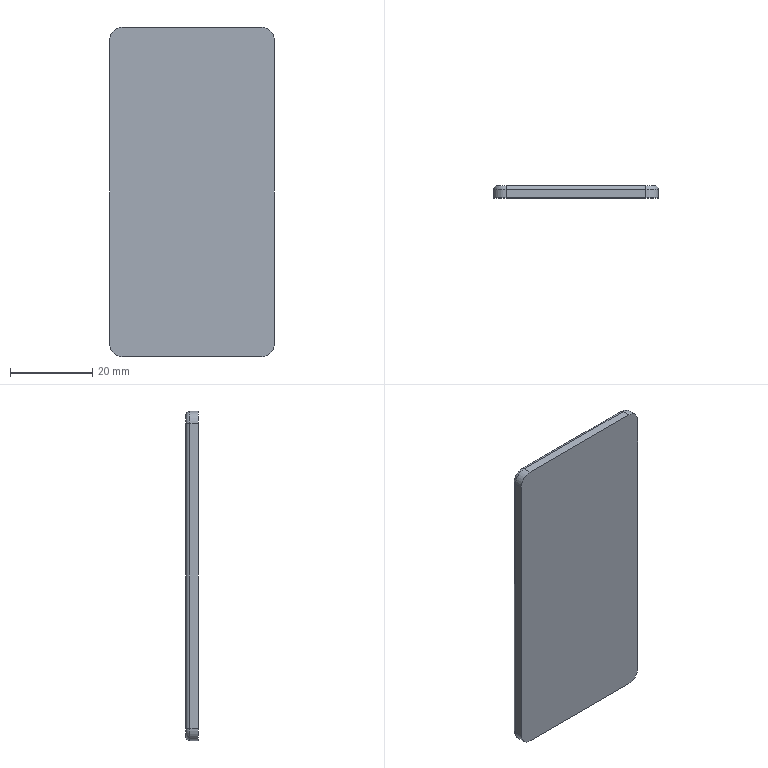Part | SolidWorks | features Fillet 2, Extrusion 1 | 1 solid | 18 faces | box 40 x 3 x 80 mm | volume 9527 mm3 | cylinder 8 | plane 6 | torus 4 | commonest cylinder face diameters 2 x4 6 x4
STEP:
#1=CARTESIAN_POINT('',(20.,0.,-37.));
#2=VERTEX_POINT('',#1);
#3=CARTESIAN_POINT('',(20.,2.,-37.));
#4=VERTEX_POINT('',#3);
#5=CARTESIAN_POINT('',(20.,3.,-37.));
#6=DIRECTION('',(0.,1.,0.));
#7=VECTOR('',#6,1000.);
#8=LINE('',#5,#7);
#9=EDGE_CURVE('',#2,#4,#8,.T.);
#10=ORIENTED_EDGE('',*,*,#9,.T.);
#11=CARTESIAN_POINT('',(20.,2.,37.));
#12=VERTEX_POINT('',#11);
#13=CARTESIAN_POINT('',(20.,2.,40.));
#14=DIRECTION('',(0.,0.,1.));
#15=VECTOR('',#14,1000.);
#16=LINE('',#13,#15);
#17=EDGE_CURVE('',#4,#12,#16,.T.);
#18=ORIENTED_EDGE('',*,*,#17,.T.);
#19=CARTESIAN_POINT('',(20.,0.,37.));
#20=VERTEX_POINT('',#19);
#21=CARTESIAN_POINT('',(20.,3.,37.));
#22=DIRECTION('',(0.,-1.,0.));
#23=VECTOR('',#22,1000.);
#24=LINE('',#21,#23);
#25=EDGE_CURVE('',#12,#20,#24,.T.);
#26=ORIENTED_EDGE('',*,*,#25,.T.);
#27=CARTESIAN_POINT('',(20.,0.,40.));
#28=DIRECTION('',(0.,0.,-1.));
#29=VECTOR('',#28,1000.);
#30=LINE('',#27,#29);
#31=EDGE_CURVE('',#20,#2,#30,.T.);
#32=ORIENTED_EDGE('',*,*,#31,.T.);
#33=EDGE_LOOP('',(#10,#18,#26,#32));
#34=FACE_OUTER_BOUND('',#33,.T.);
#35=CARTESIAN_POINT('',(20.,3.,40.));
#36=DIRECTION('',(-1.,0.,0.));
#37=DIRECTION('',(0.,0.,1.));
#38=AXIS2_PLACEMENT_3D('',#35,#36,#37);
#39=PLANE('',#38);
#40=ADVANCED_FACE('',(#34),#39,.F.);
#41=CARTESIAN_POINT('',(-17.,0.,-40.));
#42=VERTEX_POINT('',#41);
#43=CARTESIAN_POINT('',(-17.,2.,-40.));
#44=VERTEX_POINT('',#43);
#45=CARTESIAN_POINT('',(-17.,3.,-40.));
#46=DIRECTION('',(0.,1.,0.));
#47=VECTOR('',#46,1000.);
#48=LINE('',#45,#47);
#49=EDGE_CURVE('',#42,#44,#48,.T.);
#50=ORIENTED_EDGE('',*,*,#49,.T.);
#51=CARTESIAN_POINT('',(17.,2.,-40.));
#52=VERTEX_POINT('',#51);
#53=CARTESIAN_POINT('',(-20.,2.,-40.));
#54=DIRECTION('',(1.,0.,0.));
#55=VECTOR('',#54,1000.);
#56=LINE('',#53,#55);
#57=EDGE_CURVE('',#44,#52,#56,.T.);
#58=ORIENTED_EDGE('',*,*,#57,.T.);
#59=CARTESIAN_POINT('',(17.,0.,-40.));
#60=VERTEX_POINT('',#59);
#61=CARTESIAN_POINT('',(17.,3.,-40.));
#62=DIRECTION('',(0.,-1.,0.));
#63=VECTOR('',#62,1000.);
#64=LINE('',#61,#63);
#65=EDGE_CURVE('',#52,#60,#64,.T.);
#66=ORIENTED_EDGE('',*,*,#65,.T.);
#67=CARTESIAN_POINT('',(-20.,0.,-40.));
#68=DIRECTION('',(-1.,0.,0.));
#69=VECTOR('',#68,1000.);
#70=LINE('',#67,#69);
#71=EDGE_CURVE('',#60,#42,#70,.T.);
#72=ORIENTED_EDGE('',*,*,#71,.T.);
#73=EDGE_LOOP('',(#50,#58,#66,#72));
#74=FACE_OUTER_BOUND('',#73,.T.);
#75=CARTESIAN_POINT('',(-20.,3.,-40.));
#76=DIRECTION('',(0.,0.,1.));
#77=DIRECTION('',(1.,0.,0.));
#78=AXIS2_PLACEMENT_3D('',#75,#76,#77);
#79=PLANE('',#78);
#80=ADVANCED_FACE('',(#74),#79,.F.);
#81=CARTESIAN_POINT('',(-20.,0.,37.));
#82=VERTEX_POINT('',#81);
#83=CARTESIAN_POINT('',(-20.,2.,37.));
#84=VERTEX_POINT('',#83);
#85=CARTESIAN_POINT('',(-20.,3.,37.));
#86=DIRECTION('',(0.,1.,0.));
#87=VECTOR('',#86,1000.);
#88=LINE('',#85,#87);
#89=EDGE_CURVE('',#82,#84,#88,.T.);
#90=ORIENTED_EDGE('',*,*,#89,.T.);
#91=CARTESIAN_POINT('',(-20.,2.,-37.));
#92=VERTEX_POINT('',#91);
#93=CARTESIAN_POINT('',(-20.,2.,40.));
#94=DIRECTION('',(0.,0.,-1.));
#95=VECTOR('',#94,1000.);
#96=LINE('',#93,#95);
#97=EDGE_CURVE('',#84,#92,#96,.T.);
#98=ORIENTED_EDGE('',*,*,#97,.T.);
#99=CARTESIAN_POINT('',(-20.,0.,-37.));
#100=VERTEX_POINT('',#99);
#101=CARTESIAN_POINT('',(-20.,3.,-37.));
#102=DIRECTION('',(0.,-1.,0.));
#103=VECTOR('',#102,1000.);
#104=LINE('',#101,#103);
#105=EDGE_CURVE('',#92,#100,#104,.T.);
#106=ORIENTED_EDGE('',*,*,#105,.T.);
#107=CARTESIAN_POINT('',(-20.,0.,40.));
#108=DIRECTION('',(0.,0.,1.));
#109=VECTOR('',#108,1000.);
#110=LINE('',#107,#109);
#111=EDGE_CURVE('',#100,#82,#110,.T.);
#112=ORIENTED_EDGE('',*,*,#111,.T.);
#113=EDGE_LOOP('',(#90,#98,#106,#112));
#114=FACE_OUTER_BOUND('',#113,.T.);
#115=CARTESIAN_POINT('',(-20.,3.,40.));
#116=DIRECTION('',(1.,0.,0.));
#117=DIRECTION('',(0.,0.,-1.));
#118=AXIS2_PLACEMENT_3D('',#115,#116,#117);
#119=PLANE('',#118);
#120=ADVANCED_FACE('',(#114),#119,.F.);
#121=CARTESIAN_POINT('',(17.,0.,40.));
#122=VERTEX_POINT('',#121);
#123=CARTESIAN_POINT('',(17.,2.,40.));
#124=VERTEX_POINT('',#123);
#125=CARTESIAN_POINT('',(17.,3.,40.));
#126=DIRECTION('',(0.,1.,0.));
#127=VECTOR('',#126,1000.);
#128=LINE('',#125,#127);
#129=EDGE_CURVE('',#122,#124,#128,.T.);
#130=ORIENTED_EDGE('',*,*,#129,.T.);
#131=CARTESIAN_POINT('',(-17.,2.,40.));
#132=VERTEX_POINT('',#131);
#133=CARTESIAN_POINT('',(-20.,2.,40.));
#134=DIRECTION('',(-1.,0.,0.));
#135=VECTOR('',#134,1000.);
#136=LINE('',#133,#135);
#137=EDGE_CURVE('',#124,#132,#136,.T.);
#138=ORIENTED_EDGE('',*,*,#137,.T.);
#139=CARTESIAN_POINT('',(-17.,0.,40.));
#140=VERTEX_POINT('',#139);
#141=CARTESIAN_POINT('',(-17.,3.,40.));
#142=DIRECTION('',(0.,-1.,0.));
#143=VECTOR('',#142,1000.);
#144=LINE('',#141,#143);
#145=EDGE_CURVE('',#132,#140,#144,.T.);
#146=ORIENTED_EDGE('',*,*,#145,.T.);
#147=CARTESIAN_POINT('',(-20.,0.,40.));
#148=DIRECTION('',(1.,0.,0.));
#149=VECTOR('',#148,1000.);
#150=LINE('',#147,#149);
#151=EDGE_CURVE('',#140,#122,#150,.T.);
#152=ORIENTED_EDGE('',*,*,#151,.T.);
#153=EDGE_LOOP('',(#130,#138,#146,#152));
#154=FACE_OUTER_BOUND('',#153,.T.);
#155=CARTESIAN_POINT('',(-20.,3.,40.));
#156=DIRECTION('',(0.,0.,-1.));
#157=DIRECTION('',(-1.,0.,0.));
#158=AXIS2_PLACEMENT_3D('',#155,#156,#157);
#159=PLANE('',#158);
#160=ADVANCED_FACE('',(#154),#159,.F.);
#161=CARTESIAN_POINT('',(19.,3.,37.));
#162=VERTEX_POINT('',#161);
#163=CARTESIAN_POINT('',(19.,3.,-37.));
#164=VERTEX_POINT('',#163);
#165=CARTESIAN_POINT('',(19.,3.,0.));
#166=DIRECTION('',(0.,0.,-1.));
#167=VECTOR('',#166,1000.);
#168=LINE('',#165,#167);
#169=EDGE_CURVE('',#162,#164,#168,.T.);
#170=ORIENTED_EDGE('',*,*,#169,.T.);
#171=CARTESIAN_POINT('',(17.,3.,-39.));
#172=VERTEX_POINT('',#171);
#173=CARTESIAN_POINT('',(17.,3.,-37.));
#174=DIRECTION('',(0.,1.,0.));
#175=DIRECTION('',(0.,0.,-1.));
#176=AXIS2_PLACEMENT_3D('',#173,#174,#175);
#177=CIRCLE('',#176,2.);
#178=EDGE_CURVE('',#164,#172,#177,.T.);
#179=ORIENTED_EDGE('',*,*,#178,.T.);
#180=CARTESIAN_POINT('',(-17.,3.,-39.));
#181=VERTEX_POINT('',#180);
#182=CARTESIAN_POINT('',(0.,3.,-39.));
#183=DIRECTION('',(-1.,0.,0.));
#184=VECTOR('',#183,1000.);
#185=LINE('',#182,#184);
#186=EDGE_CURVE('',#172,#181,#185,.T.);
#187=ORIENTED_EDGE('',*,*,#186,.T.);
#188=CARTESIAN_POINT('',(-19.,3.,-37.));
#189=VERTEX_POINT('',#188);
#190=CARTESIAN_POINT('',(-17.,3.,-37.));
#191=DIRECTION('',(0.,1.,0.));
#192=DIRECTION('',(0.,0.,-1.));
#193=AXIS2_PLACEMENT_3D('',#190,#191,#192);
#194=CIRCLE('',#193,2.);
#195=EDGE_CURVE('',#181,#189,#194,.T.);
#196=ORIENTED_EDGE('',*,*,#195,.T.);
#197=CARTESIAN_POINT('',(-19.,3.,37.));
#198=VERTEX_POINT('',#197);
#199=CARTESIAN_POINT('',(-19.,3.,0.));
#200=DIRECTION('',(0.,0.,1.));
#201=VECTOR('',#200,1000.);
#202=LINE('',#199,#201);
#203=EDGE_CURVE('',#189,#198,#202,.T.);
#204=ORIENTED_EDGE('',*,*,#203,.T.);
#205=CARTESIAN_POINT('',(-17.,3.,39.));
#206=VERTEX_POINT('',#205);
#207=CARTESIAN_POINT('',(-17.,3.,37.));
#208=DIRECTION('',(0.,1.,0.));
#209=DIRECTION('',(0.,0.,-1.));
#210=AXIS2_PLACEMENT_3D('',#207,#208,#209);
#211=CIRCLE('',#210,2.);
#212=EDGE_CURVE('',#198,#206,#211,.T.);
#213=ORIENTED_EDGE('',*,*,#212,.T.);
#214=CARTESIAN_POINT('',(17.,3.,39.));
#215=VERTEX_POINT('',#214);
#216=CARTESIAN_POINT('',(0.,3.,39.));
#217=DIRECTION('',(1.,0.,0.));
#218=VECTOR('',#217,1000.);
#219=LINE('',#216,#218);
#220=EDGE_CURVE('',#206,#215,#219,.T.);
#221=ORIENTED_EDGE('',*,*,#220,.T.);
#222=CARTESIAN_POINT('',(17.,3.,37.));
#223=DIRECTION('',(0.,1.,0.));
#224=DIRECTION('',(0.,0.,-1.));
#225=AXIS2_PLACEMENT_3D('',#222,#223,#224);
#226=CIRCLE('',#225,2.);
#227=EDGE_CURVE('',#215,#162,#226,.T.);
#228=ORIENTED_EDGE('',*,*,#227,.T.);
#229=EDGE_LOOP('',(#170,#179,#187,#196,#204,#213,#221,#228));
#230=FACE_OUTER_BOUND('',#229,.T.);
#231=CARTESIAN_POINT('',(0.,3.,0.));
#232=DIRECTION('',(0.,-1.,0.));
#233=DIRECTION('',(0.,0.,-1.));
#234=AXIS2_PLACEMENT_3D('',#231,#232,#233);
#235=PLANE('',#234);
#236=ADVANCED_FACE('',(#230),#235,.F.);
#237=ORIENTED_EDGE('',*,*,#111,.F.);
#238=CARTESIAN_POINT('',(-17.,0.,-37.));
#239=DIRECTION('',(0.,-1.,0.));
#240=DIRECTION('',(0.,0.,-1.));
#241=AXIS2_PLACEMENT_3D('',#238,#239,#240);
#242=CIRCLE('',#241,3.);
#243=EDGE_CURVE('',#100,#42,#242,.T.);
#244=ORIENTED_EDGE('',*,*,#243,.T.);
#245=ORIENTED_EDGE('',*,*,#71,.F.);
#246=CARTESIAN_POINT('',(17.,0.,-37.));
#247=DIRECTION('',(0.,-1.,0.));
#248=DIRECTION('',(0.,0.,-1.));
#249=AXIS2_PLACEMENT_3D('',#246,#247,#248);
#250=CIRCLE('',#249,3.);
#251=EDGE_CURVE('',#60,#2,#250,.T.);
#252=ORIENTED_EDGE('',*,*,#251,.T.);
#253=ORIENTED_EDGE('',*,*,#31,.F.);
#254=CARTESIAN_POINT('',(17.,0.,37.));
#255=DIRECTION('',(0.,-1.,0.));
#256=DIRECTION('',(0.,0.,-1.));
#257=AXIS2_PLACEMENT_3D('',#254,#255,#256);
#258=CIRCLE('',#257,3.);
#259=EDGE_CURVE('',#20,#122,#258,.T.);
#260=ORIENTED_EDGE('',*,*,#259,.T.);
#261=ORIENTED_EDGE('',*,*,#151,.F.);
#262=CARTESIAN_POINT('',(-17.,0.,37.));
#263=DIRECTION('',(0.,-1.,0.));
#264=DIRECTION('',(0.,0.,-1.));
#265=AXIS2_PLACEMENT_3D('',#262,#263,#264);
#266=CIRCLE('',#265,3.);
#267=EDGE_CURVE('',#140,#82,#266,.T.);
#268=ORIENTED_EDGE('',*,*,#267,.T.);
#269=EDGE_LOOP('',(#237,#244,#245,#252,#253,#260,#261,#268));
#270=FACE_OUTER_BOUND('',#269,.T.);
#271=CARTESIAN_POINT('',(0.,0.,0.));
#272=DIRECTION('',(0.,-1.,0.));
#273=DIRECTION('',(0.,0.,-1.));
#274=AXIS2_PLACEMENT_3D('',#271,#272,#273);
#275=PLANE('',#274);
#276=ADVANCED_FACE('',(#270),#275,.T.);
#277=ORIENTED_EDGE('',*,*,#105,.F.);
#278=CARTESIAN_POINT('',(-17.,2.,-37.));
#279=DIRECTION('',(0.,-1.,0.));
#280=DIRECTION('',(0.,0.,-1.));
#281=AXIS2_PLACEMENT_3D('',#278,#279,#280);
#282=CIRCLE('',#281,3.);
#283=EDGE_CURVE('',#92,#44,#282,.T.);
#284=ORIENTED_EDGE('',*,*,#283,.T.);
#285=ORIENTED_EDGE('',*,*,#49,.F.);
#286=ORIENTED_EDGE('',*,*,#243,.F.);
#287=EDGE_LOOP('',(#277,#284,#285,#286));
#288=FACE_OUTER_BOUND('',#287,.T.);
#289=CARTESIAN_POINT('',(-17.,3.,-37.));
#290=DIRECTION('',(0.,-1.,0.));
#291=DIRECTION('',(0.,0.,-1.));
#292=AXIS2_PLACEMENT_3D('',#289,#290,#291);
#293=CYLINDRICAL_SURFACE('',#292,3.);
#294=ADVANCED_FACE('',(#288),#293,.T.);
#295=ORIENTED_EDGE('',*,*,#65,.F.);
#296=CARTESIAN_POINT('',(17.,2.,-37.));
#297=DIRECTION('',(0.,-1.,0.));
#298=DIRECTION('',(0.,0.,-1.));
#299=AXIS2_PLACEMENT_3D('',#296,#297,#298);
#300=CIRCLE('',#299,3.);
#301=EDGE_CURVE('',#52,#4,#300,.T.);
#302=ORIENTED_EDGE('',*,*,#301,.T.);
#303=ORIENTED_EDGE('',*,*,#9,.F.);
#304=ORIENTED_EDGE('',*,*,#251,.F.);
#305=EDGE_LOOP('',(#295,#302,#303,#304));
#306=FACE_OUTER_BOUND('',#305,.T.);
#307=CARTESIAN_POINT('',(17.,3.,-37.));
#308=DIRECTION('',(0.,-1.,0.));
#309=DIRECTION('',(0.,0.,-1.));
#310=AXIS2_PLACEMENT_3D('',#307,#308,#309);
#311=CYLINDRICAL_SURFACE('',#310,3.);
#312=ADVANCED_FACE('',(#306),#311,.T.);
#313=ORIENTED_EDGE('',*,*,#145,.F.);
#314=CARTESIAN_POINT('',(-17.,2.,37.));
#315=DIRECTION('',(0.,-1.,0.));
#316=DIRECTION('',(0.,0.,-1.));
#317=AXIS2_PLACEMENT_3D('',#314,#315,#316);
#318=CIRCLE('',#317,3.);
#319=EDGE_CURVE('',#132,#84,#318,.T.);
#320=ORIENTED_EDGE('',*,*,#319,.T.);
#321=ORIENTED_EDGE('',*,*,#89,.F.);
#322=ORIENTED_EDGE('',*,*,#267,.F.);
#323=EDGE_LOOP('',(#313,#320,#321,#322));
#324=FACE_OUTER_BOUND('',#323,.T.);
#325=CARTESIAN_POINT('',(-17.,3.,37.));
#326=DIRECTION('',(0.,-1.,0.));
#327=DIRECTION('',(0.,0.,-1.));
#328=AXIS2_PLACEMENT_3D('',#325,#326,#327);
#329=CYLINDRICAL_SURFACE('',#328,3.);
#330=ADVANCED_FACE('',(#324),#329,.T.);
#331=ORIENTED_EDGE('',*,*,#25,.F.);
#332=CARTESIAN_POINT('',(17.,2.,37.));
#333=DIRECTION('',(0.,-1.,0.));
#334=DIRECTION('',(0.,0.,-1.));
#335=AXIS2_PLACEMENT_3D('',#332,#333,#334);
#336=CIRCLE('',#335,3.);
#337=EDGE_CURVE('',#12,#124,#336,.T.);
#338=ORIENTED_EDGE('',*,*,#337,.T.);
#339=ORIENTED_EDGE('',*,*,#129,.F.);
#340=ORIENTED_EDGE('',*,*,#259,.F.);
#341=EDGE_LOOP('',(#331,#338,#339,#340));
#342=FACE_OUTER_BOUND('',#341,.T.);
#343=CARTESIAN_POINT('',(17.,3.,37.));
#344=DIRECTION('',(0.,-1.,0.));
#345=DIRECTION('',(0.,0.,-1.));
#346=AXIS2_PLACEMENT_3D('',#343,#344,#345);
#347=CYLINDRICAL_SURFACE('',#346,3.);
#348=ADVANCED_FACE('',(#342),#347,.T.);
#349=CARTESIAN_POINT('',(-19.,2.,37.));
#350=DIRECTION('',(0.,0.,-1.));
#351=DIRECTION('',(-1.,0.,0.));
#352=AXIS2_PLACEMENT_3D('',#349,#350,#351);
#353=CIRCLE('',#352,1.);
#354=EDGE_CURVE('',#84,#198,#353,.T.);
#355=ORIENTED_EDGE('',*,*,#354,.F.);
#356=ORIENTED_EDGE('',*,*,#319,.F.);
#357=CARTESIAN_POINT('',(-17.,2.,39.));
#358=DIRECTION('',(1.,0.,0.));
#359=DIRECTION('',(0.,0.,-1.));
#360=AXIS2_PLACEMENT_3D('',#357,#358,#359);
#361=CIRCLE('',#360,1.);
#362=EDGE_CURVE('',#206,#132,#361,.T.);
#363=ORIENTED_EDGE('',*,*,#362,.F.);
#364=ORIENTED_EDGE('',*,*,#212,.F.);
#365=EDGE_LOOP('',(#355,#356,#363,#364));
#366=FACE_OUTER_BOUND('',#365,.T.);
#367=CARTESIAN_POINT('',(-17.,2.,37.));
#368=DIRECTION('',(0.,-1.,0.));
#369=DIRECTION('',(0.,0.,-1.));
#370=AXIS2_PLACEMENT_3D('',#367,#368,#369);
#371=TOROIDAL_SURFACE('',#370,2.,1.);
#372=ADVANCED_FACE('',(#366),#371,.T.);
#373=ORIENTED_EDGE('',*,*,#362,.T.);
#374=ORIENTED_EDGE('',*,*,#137,.F.);
#375=CARTESIAN_POINT('',(17.,2.,39.));
#376=DIRECTION('',(1.,0.,0.));
#377=DIRECTION('',(0.,0.,-1.));
#378=AXIS2_PLACEMENT_3D('',#375,#376,#377);
#379=CIRCLE('',#378,1.);
#380=EDGE_CURVE('',#215,#124,#379,.T.);
#381=ORIENTED_EDGE('',*,*,#380,.F.);
#382=ORIENTED_EDGE('',*,*,#220,.F.);
#383=EDGE_LOOP('',(#373,#374,#381,#382));
#384=FACE_OUTER_BOUND('',#383,.T.);
#385=CARTESIAN_POINT('',(0.,2.,39.));
#386=DIRECTION('',(1.,0.,0.));
#387=DIRECTION('',(0.,0.,-1.));
#388=AXIS2_PLACEMENT_3D('',#385,#386,#387);
#389=CYLINDRICAL_SURFACE('',#388,1.);
#390=ADVANCED_FACE('',(#384),#389,.T.);
#391=ORIENTED_EDGE('',*,*,#354,.T.);
#392=ORIENTED_EDGE('',*,*,#203,.F.);
#393=CARTESIAN_POINT('',(-19.,2.,-37.));
#394=DIRECTION('',(0.,0.,-1.));
#395=DIRECTION('',(-1.,0.,0.));
#396=AXIS2_PLACEMENT_3D('',#393,#394,#395);
#397=CIRCLE('',#396,1.);
#398=EDGE_CURVE('',#92,#189,#397,.T.);
#399=ORIENTED_EDGE('',*,*,#398,.F.);
#400=ORIENTED_EDGE('',*,*,#97,.F.);
#401=EDGE_LOOP('',(#391,#392,#399,#400));
#402=FACE_OUTER_BOUND('',#401,.T.);
#403=CARTESIAN_POINT('',(-19.,2.,0.));
#404=DIRECTION('',(0.,0.,1.));
#405=DIRECTION('',(1.,0.,0.));
#406=AXIS2_PLACEMENT_3D('',#403,#404,#405);
#407=CYLINDRICAL_SURFACE('',#406,1.);
#408=ADVANCED_FACE('',(#402),#407,.T.);
#409=ORIENTED_EDGE('',*,*,#380,.T.);
#410=ORIENTED_EDGE('',*,*,#337,.F.);
#411=CARTESIAN_POINT('',(19.,2.,37.));
#412=DIRECTION('',(0.,0.,-1.));
#413=DIRECTION('',(-1.,0.,0.));
#414=AXIS2_PLACEMENT_3D('',#411,#412,#413);
#415=CIRCLE('',#414,1.);
#416=EDGE_CURVE('',#162,#12,#415,.T.);
#417=ORIENTED_EDGE('',*,*,#416,.F.);
#418=ORIENTED_EDGE('',*,*,#227,.F.);
#419=EDGE_LOOP('',(#409,#410,#417,#418));
#420=FACE_OUTER_BOUND('',#419,.T.);
#421=CARTESIAN_POINT('',(17.,2.,37.));
#422=DIRECTION('',(0.,-1.,0.));
#423=DIRECTION('',(0.,0.,-1.));
#424=AXIS2_PLACEMENT_3D('',#421,#422,#423);
#425=TOROIDAL_SURFACE('',#424,2.,1.);
#426=ADVANCED_FACE('',(#420),#425,.T.);
#427=ORIENTED_EDGE('',*,*,#398,.T.);
#428=ORIENTED_EDGE('',*,*,#195,.F.);
#429=CARTESIAN_POINT('',(-17.,2.,-39.));
#430=DIRECTION('',(1.,0.,0.));
#431=DIRECTION('',(0.,0.,-1.));
#432=AXIS2_PLACEMENT_3D('',#429,#430,#431);
#433=CIRCLE('',#432,1.);
#434=EDGE_CURVE('',#44,#181,#433,.T.);
#435=ORIENTED_EDGE('',*,*,#434,.F.);
#436=ORIENTED_EDGE('',*,*,#283,.F.);
#437=EDGE_LOOP('',(#427,#428,#435,#436));
#438=FACE_OUTER_BOUND('',#437,.T.);
#439=CARTESIAN_POINT('',(-17.,2.,-37.));
#440=DIRECTION('',(0.,-1.,0.));
#441=DIRECTION('',(0.,0.,-1.));
#442=AXIS2_PLACEMENT_3D('',#439,#440,#441);
#443=TOROIDAL_SURFACE('',#442,2.,1.);
#444=ADVANCED_FACE('',(#438),#443,.T.);
#445=ORIENTED_EDGE('',*,*,#416,.T.);
#446=ORIENTED_EDGE('',*,*,#17,.F.);
#447=CARTESIAN_POINT('',(19.,2.,-37.));
#448=DIRECTION('',(0.,0.,-1.));
#449=DIRECTION('',(-1.,0.,0.));
#450=AXIS2_PLACEMENT_3D('',#447,#448,#449);
#451=CIRCLE('',#450,1.);
#452=EDGE_CURVE('',#164,#4,#451,.T.);
#453=ORIENTED_EDGE('',*,*,#452,.F.);
#454=ORIENTED_EDGE('',*,*,#169,.F.);
#455=EDGE_LOOP('',(#445,#446,#453,#454));
#456=FACE_OUTER_BOUND('',#455,.T.);
#457=CARTESIAN_POINT('',(19.,2.,0.));
#458=DIRECTION('',(0.,0.,-1.));
#459=DIRECTION('',(-1.,0.,0.));
#460=AXIS2_PLACEMENT_3D('',#457,#458,#459);
#461=CYLINDRICAL_SURFACE('',#460,1.);
#462=ADVANCED_FACE('',(#456),#461,.T.);
#463=ORIENTED_EDGE('',*,*,#434,.T.);
#464=ORIENTED_EDGE('',*,*,#186,.F.);
#465=CARTESIAN_POINT('',(17.,2.,-39.));
#466=DIRECTION('',(1.,0.,0.));
#467=DIRECTION('',(0.,0.,-1.));
#468=AXIS2_PLACEMENT_3D('',#465,#466,#467);
#469=CIRCLE('',#468,1.);
#470=EDGE_CURVE('',#52,#172,#469,.T.);
#471=ORIENTED_EDGE('',*,*,#470,.F.);
#472=ORIENTED_EDGE('',*,*,#57,.F.);
#473=EDGE_LOOP('',(#463,#464,#471,#472));
#474=FACE_OUTER_BOUND('',#473,.T.);
#475=CARTESIAN_POINT('',(0.,2.,-39.));
#476=DIRECTION('',(-1.,0.,0.));
#477=DIRECTION('',(0.,0.,1.));
#478=AXIS2_PLACEMENT_3D('',#475,#476,#477);
#479=CYLINDRICAL_SURFACE('',#478,1.);
#480=ADVANCED_FACE('',(#474),#479,.T.);
#481=ORIENTED_EDGE('',*,*,#452,.T.);
#482=ORIENTED_EDGE('',*,*,#301,.F.);
#483=ORIENTED_EDGE('',*,*,#470,.T.);
#484=ORIENTED_EDGE('',*,*,#178,.F.);
#485=EDGE_LOOP('',(#481,#482,#483,#484));
#486=FACE_OUTER_BOUND('',#485,.T.);
#487=CARTESIAN_POINT('',(17.,2.,-37.));
#488=DIRECTION('',(0.,-1.,0.));
#489=DIRECTION('',(0.,0.,-1.));
#490=AXIS2_PLACEMENT_3D('',#487,#488,#489);
#491=TOROIDAL_SURFACE('',#490,2.,1.);
#492=ADVANCED_FACE('',(#486),#491,.T.);
#493=CLOSED_SHELL('',(#40,#80,#120,#160,#236,#276,#294,#312,#330,#348,#372,#390,#408,#426,#444,#462,#480,#492));
#494=MANIFOLD_SOLID_BREP('',#493);
#495=CARTESIAN_POINT('',(0.,0.,0.));
#496=DIRECTION('',(0.,0.,1.));
#497=DIRECTION('',(1.,0.,0.));
#498=AXIS2_PLACEMENT_3D('',#495,#496,#497);
#499=(LENGTH_UNIT()NAMED_UNIT(*)SI_UNIT(.MILLI.,.METRE.));
#500=UNCERTAINTY_MEASURE_WITH_UNIT(LENGTH_MEASURE(0.00001),#499,'','');
#501=(NAMED_UNIT(*)PLANE_ANGLE_UNIT()SI_UNIT($,.RADIAN.));
#502=(NAMED_UNIT(*)SI_UNIT($,.STERADIAN.)SOLID_ANGLE_UNIT());
#503=(GEOMETRIC_REPRESENTATION_CONTEXT(3)GLOBAL_UNCERTAINTY_ASSIGNED_CONTEXT((#500))GLOBAL_UNIT_ASSIGNED_CONTEXT((#499,#501,#502))REPRESENTATION_CONTEXT('',''));
#504=ADVANCED_BREP_SHAPE_REPRESENTATION('',(#494,#498),#503);